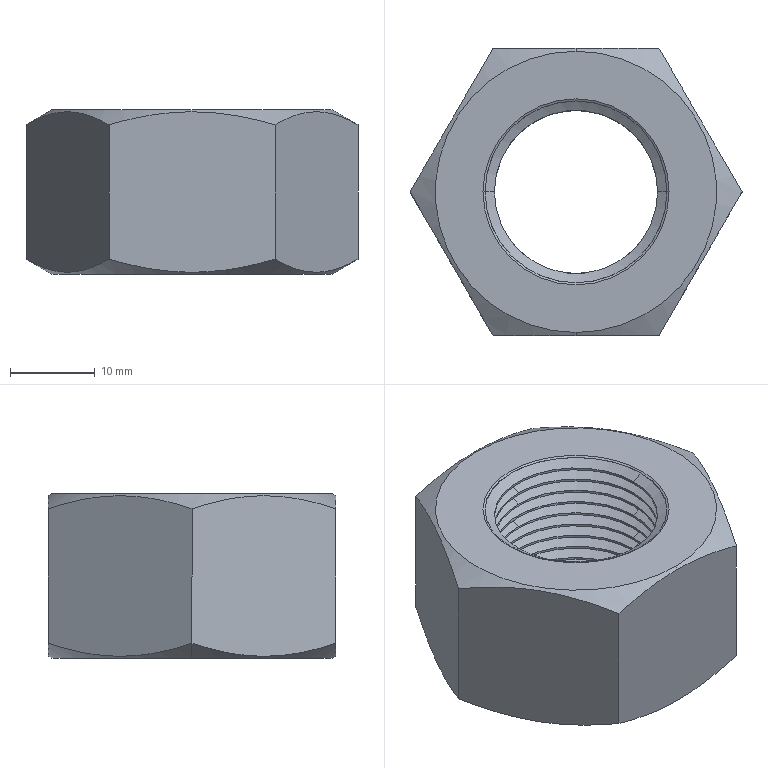Part | SolidWorks | features BaseBody 1 | 1 solid | 86 faces | box 39.26 x 34 x 19.4 mm | volume 12999 mm3 | cone 56 | cylinder 22 | plane 8 | commonest cylinder face diameters 19.294 x22